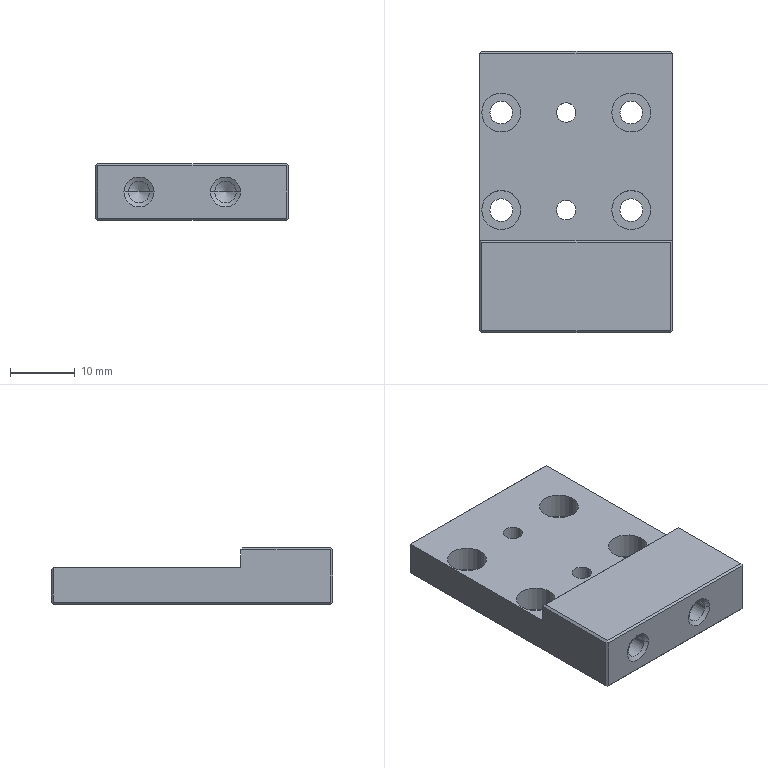Part | NX | 1 solid | 61 faces | box 29.6 x 43.24 x 8.65 mm | volume 7661 mm3 | cylinder 28 | plane 25 | cone 8 | commonest cylinder face diameters 3.3 x8 3.5 x8 6 x8 3 x4